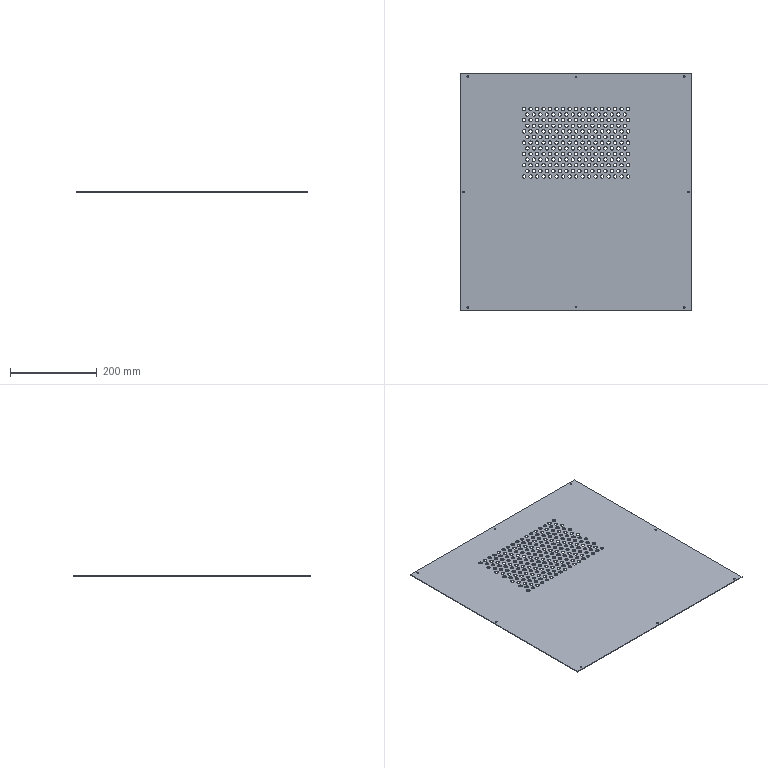Part | STEP file | x77-05102 | 1 solid | 452 faces | box 535 x 548 x 1.5 mm | volume 423444 mm3 | cylinder 446 | plane 6 | commonest cylinder face diameters 8 x430 3.5 x16